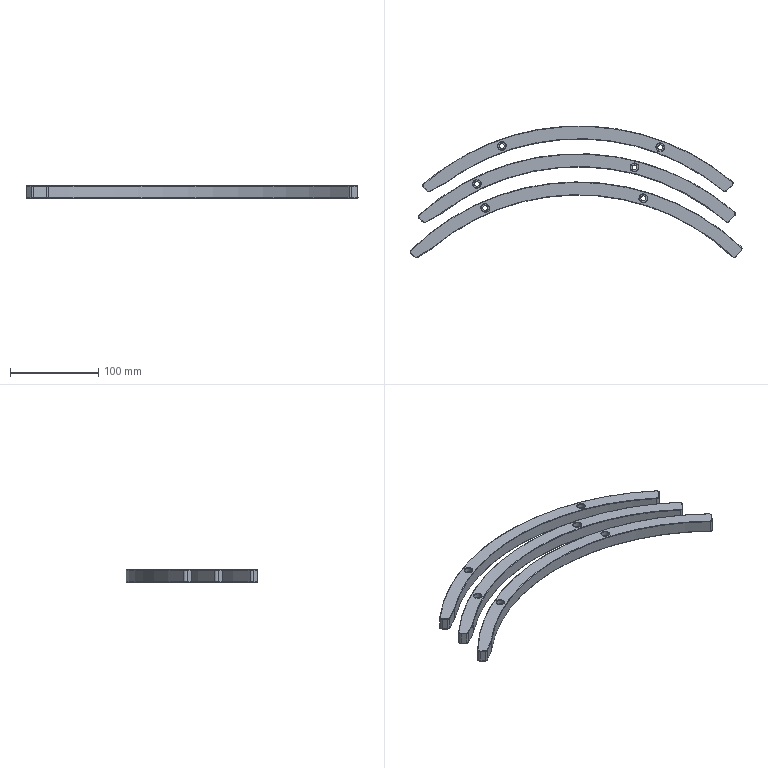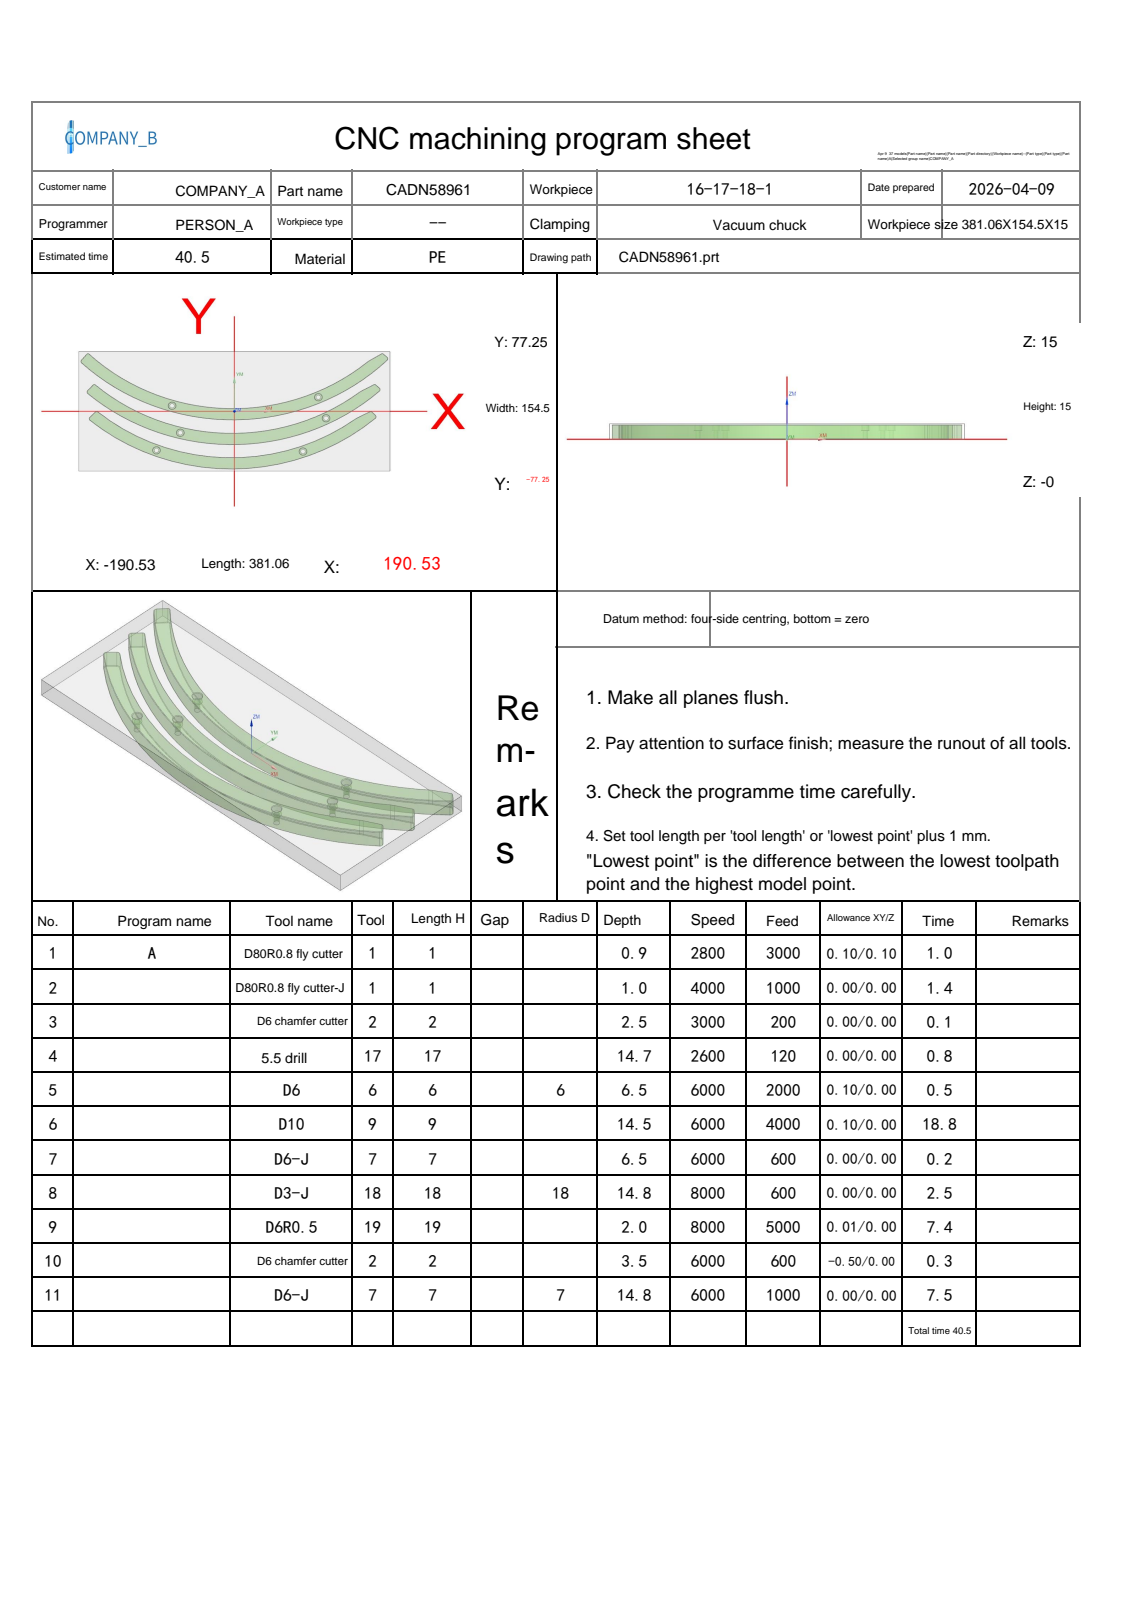NC program | NX | posted by the shop | part box 376.065 x 149.521 x 14 mm
Lines 357 to 1635 of 3929, first 1032 of 1279 lines:
N6 T09 M06
(D10  D=10. R=0. H=09 ce=0.10 di=0.00)
(MAX_Z=34. MIN_Z=0.5 Time=18.78M)
G00 G90 G54 X168.192 Y73.348 M03 S6000
G43 H09 Z34.
M08
Z14.5
G01 X177.404 Y78.848 Z14.494 F4000.
G02 X185.678 Y78.13 Z14.489 I3.64 J-6.096
G01 X190.32 Y74.13 Z14.486
G02 X191.169 Y62.707 Z14.479 I-5.287 J-6.136
X190.701 Y62.208 Z14.478 I-6.136 J5.287
X-11.247 Y-16.23 Z14.355 I-192.53 J196.5
X-190.59 Y58.586 Z14.245 I9.419 J274.939
X-191.169 Y69.766 Z14.238 I5.558 J5.892
G01 X-184.602 Y77.387 Z14.232
G02 X-174.589 Y78.131 Z14.226 I5.379 J-4.635
X-174.323 Y77.889 Z14.226 I-4.635 J-5.379
G03 X159.163 Y67.576 Z14.023 I172.494 J180.819
G02 X162.467 Y69.93 Z14.021 I16.17 J-19.197
G01 X177.404 Y78.848 Z14.011
G02 X185.678 Y78.13 Z14.006 I3.64 J-6.096
G01 X190.32 Y74.13 Z14.003
G02 X191.169 Y62.707 Z13.996 I-5.287 J-6.136
X190.701 Y62.208 Z13.996 I-6.136 J5.287
X-11.247 Y-16.23 Z13.872 I-192.53 J196.5
X-190.59 Y58.586 Z13.762 I9.419 J274.939
X-191.169 Y69.766 Z13.755 I5.558 J5.892
G01 X-184.602 Y77.387 Z13.749
G02 X-174.589 Y78.131 Z13.743 I5.379 J-4.635
X-174.323 Y77.889 Z13.743 I-4.635 J-5.379
G03 X159.163 Y67.576 Z13.54 I172.494 J180.819
G02 X162.467 Y69.93 Z13.538 I16.17 J-19.197
G01 X177.404 Y78.848 Z13.529
G02 X185.678 Y78.13 Z13.524 I3.64 J-6.096
G01 X190.32 Y74.13 Z13.52
G02 X191.169 Y62.707 Z13.513 I-5.287 J-6.136
X190.701 Y62.208 Z13.513 I-6.136 J5.287
X-11.247 Y-16.23 Z13.389 I-192.53 J196.5
X-190.59 Y58.586 Z13.279 I9.419 J274.939
X-191.169 Y69.766 Z13.272 I5.558 J5.892
G01 X-184.602 Y77.387 Z13.267
G02 X-174.589 Y78.131 Z13.26 I5.379 J-4.635
X-174.323 Y77.889 Z13.26 I-4.635 J-5.379
G03 X159.163 Y67.576 Z13.058 I172.494 J180.819
G02 X162.467 Y69.93 Z13.055 I16.17 J-19.197
G01 X177.404 Y78.848 Z13.046
G02 X185.678 Y78.13 Z13.041 I3.64 J-6.096
G01 X190.32 Y74.13 Z13.037
G02 X191.169 Y62.707 Z13.03 I-5.287 J-6.136
X190.701 Y62.208 Z13.03 I-6.136 J5.287
X-11.247 Y-16.23 Z12.907 I-192.53 J196.5
X-190.59 Y58.586 Z12.796 I9.419 J274.939
X-191.169 Y69.766 Z12.79 I5.558 J5.892
G01 X-184.602 Y77.387 Z12.784
G02 X-174.589 Y78.131 Z12.778 I5.379 J-4.635
X-174.323 Y77.889 Z12.778 I-4.635 J-5.379
G03 X159.163 Y67.576 Z12.575 I172.494 J180.819
G02 X162.467 Y69.93 Z12.573 I16.17 J-19.197
G01 X177.404 Y78.848 Z12.563
G02 X185.678 Y78.13 Z12.558 I3.64 J-6.096
G01 X190.32 Y74.13 Z12.555
G02 X191.169 Y62.707 Z12.548 I-5.287 J-6.136
X190.701 Y62.208 Z12.547 I-6.136 J5.287
X-11.247 Y-16.23 Z12.424 I-192.53 J196.5
X-190.59 Y58.586 Z12.314 I9.419 J274.939
X-191.169 Y69.766 Z12.307 I5.558 J5.892
G01 X-184.602 Y77.387 Z12.301
G02 X-174.589 Y78.131 Z12.295 I5.379 J-4.635
X-174.323 Y77.889 Z12.295 I-4.635 J-5.379
G03 X159.163 Y67.576 Z12.092 I172.494 J180.819
G02 X162.467 Y69.93 Z12.09 I16.17 J-19.197
G01 X177.404 Y78.848 Z12.08
G02 X185.678 Y78.13 Z12.075 I3.64 J-6.096
G01 X190.32 Y74.13 Z12.072
G02 X191.169 Y62.707 Z12.065 I-5.287 J-6.136
X190.701 Y62.208 Z12.065 I-6.136 J5.287
X-11.247 Y-16.23 Z11.941 I-192.53 J196.5
X-190.59 Y58.586 Z11.831 I9.419 J274.939
X-191.169 Y69.766 Z11.824 I5.558 J5.892
G01 X-184.602 Y77.387 Z11.818
G02 X-174.589 Y78.131 Z11.812 I5.379 J-4.635
X-174.323 Y77.889 Z11.812 I-4.635 J-5.379
G03 X159.163 Y67.576 Z11.609 I172.494 J180.819
G02 X162.467 Y69.93 Z11.607 I16.17 J-19.197
G01 X177.404 Y78.848 Z11.597
G02 X185.678 Y78.13 Z11.593 I3.64 J-6.096
G01 X190.32 Y74.13 Z11.589
G02 X191.169 Y62.707 Z11.582 I-5.287 J-6.136
X190.701 Y62.208 Z11.582 I-6.136 J5.287
X-11.247 Y-16.23 Z11.458 I-192.53 J196.5
X-190.59 Y58.586 Z11.348 I9.419 J274.939
X-191.169 Y69.766 Z11.341 I5.558 J5.892
G01 X-184.602 Y77.387 Z11.336
G02 X-174.589 Y78.131 Z11.329 I5.379 J-4.635
X-174.323 Y77.889 Z11.329 I-4.635 J-5.379
G03 X159.163 Y67.576 Z11.127 I172.494 J180.819
G02 X162.467 Y69.93 Z11.124 I16.17 J-19.197
G01 X177.404 Y78.848 Z11.115
G02 X185.678 Y78.13 Z11.11 I3.64 J-6.096
G01 X190.32 Y74.13 Z11.106
G02 X191.169 Y62.707 Z11.099 I-5.287 J-6.136
X190.701 Y62.208 Z11.099 I-6.136 J5.287
X-11.247 Y-16.23 Z10.975 I-192.53 J196.5
X-190.59 Y58.586 Z10.865 I9.419 J274.939
X-191.169 Y69.766 Z10.858 I5.558 J5.892
G01 X-184.602 Y77.387 Z10.853
G02 X-174.589 Y78.131 Z10.847 I5.379 J-4.635
X-174.323 Y77.889 Z10.847 I-4.635 J-5.379
G03 X159.163 Y67.576 Z10.644 I172.494 J180.819
G02 X162.467 Y69.93 Z10.642 I16.17 J-19.197
G01 X177.404 Y78.848 Z10.632
G02 X185.678 Y78.13 Z10.627 I3.64 J-6.096
G01 X190.32 Y74.13 Z10.624
G02 X191.169 Y62.707 Z10.617 I-5.287 J-6.136
X190.701 Y62.208 Z10.616 I-6.136 J5.287
X-11.247 Y-16.23 Z10.493 I-192.53 J196.5
X-190.59 Y58.586 Z10.383 I9.419 J274.939
X-191.169 Y69.766 Z10.376 I5.558 J5.892
G01 X-184.602 Y77.387 Z10.37
G02 X-174.589 Y78.131 Z10.364 I5.379 J-4.635
X-174.323 Y77.889 Z10.364 I-4.635 J-5.379
G03 X159.163 Y67.576 Z10.161 I172.494 J180.819
G02 X162.467 Y69.93 Z10.159 I16.17 J-19.197
G01 X177.404 Y78.848 Z10.149
G02 X185.678 Y78.13 Z10.144 I3.64 J-6.096
G01 X190.32 Y74.13 Z10.141
G02 X191.169 Y62.707 Z10.134 I-5.287 J-6.136
X190.701 Y62.208 Z10.133 I-6.136 J5.287
X-11.247 Y-16.23 Z10.01 I-192.53 J196.5
X-190.59 Y58.586 Z9.9 I9.419 J274.939
X-191.169 Y69.766 Z9.893 I5.558 J5.892
G01 X-184.602 Y77.387 Z9.887
G02 X-174.589 Y78.131 Z9.881 I5.379 J-4.635
X-174.323 Y77.889 Z9.881 I-4.635 J-5.379
G03 X159.163 Y67.576 Z9.678 I172.494 J180.819
G02 X162.467 Y69.93 Z9.676 I16.17 J-19.197
G01 X177.404 Y78.848 Z9.666
G02 X185.678 Y78.13 Z9.662 I3.64 J-6.096
G01 X190.32 Y74.13 Z9.658
G02 X191.169 Y62.707 Z9.651 I-5.287 J-6.136
X190.701 Y62.208 Z9.651 I-6.136 J5.287
X-11.247 Y-16.23 Z9.527 I-192.53 J196.5
X-190.59 Y58.586 Z9.417 I9.419 J274.939
X-191.169 Y69.766 Z9.41 I5.558 J5.892
G01 X-184.602 Y77.387 Z9.405
G02 X-174.589 Y78.131 Z9.398 I5.379 J-4.635
X-174.323 Y77.889 Z9.398 I-4.635 J-5.379
G03 X159.163 Y67.576 Z9.196 I172.494 J180.819
G02 X162.467 Y69.93 Z9.193 I16.17 J-19.197
G01 X177.404 Y78.848 Z9.184
G02 X185.678 Y78.13 Z9.179 I3.64 J-6.096
G01 X190.32 Y74.13 Z9.175
G02 X191.169 Y62.707 Z9.168 I-5.287 J-6.136
X190.701 Y62.208 Z9.168 I-6.136 J5.287
X-11.247 Y-16.23 Z9.044 I-192.53 J196.5
X-190.59 Y58.586 Z8.934 I9.419 J274.939
X-191.169 Y69.766 Z8.927 I5.558 J5.892
G01 X-184.602 Y77.387 Z8.922
G02 X-174.589 Y78.131 Z8.916 I5.379 J-4.635
X-174.323 Y77.889 Z8.915 I-4.635 J-5.379
G03 X159.163 Y67.576 Z8.713 I172.494 J180.819
G02 X162.467 Y69.93 Z8.711 I16.17 J-19.197
G01 X177.404 Y78.848 Z8.701
G02 X185.678 Y78.13 Z8.696 I3.64 J-6.096
G01 X190.32 Y74.13 Z8.693
G02 X191.169 Y62.707 Z8.686 I-5.287 J-6.136
X190.701 Y62.208 Z8.685 I-6.136 J5.287
X-11.247 Y-16.23 Z8.562 I-192.53 J196.5
X-190.59 Y58.586 Z8.452 I9.419 J274.939
X-191.169 Y69.766 Z8.445 I5.558 J5.892
G01 X-184.602 Y77.387 Z8.439
G02 X-174.589 Y78.131 Z8.433 I5.379 J-4.635
X-174.323 Y77.889 Z8.433 I-4.635 J-5.379
G03 X159.163 Y67.576 Z8.23 I172.494 J180.819
G02 X162.467 Y69.93 Z8.228 I16.17 J-19.197
G01 X177.404 Y78.848 Z8.218
G02 X185.678 Y78.13 Z8.213 I3.64 J-6.096
G01 X190.32 Y74.13 Z8.21
G02 X191.169 Y62.707 Z8.203 I-5.287 J-6.136
X190.701 Y62.208 Z8.202 I-6.136 J5.287
X-11.247 Y-16.23 Z8.079 I-192.53 J196.5
X-190.59 Y58.586 Z7.969 I9.419 J274.939
X-191.169 Y69.766 Z7.962 I5.558 J5.892
G01 X-184.602 Y77.387 Z7.956
G02 X-174.589 Y78.131 Z7.95 I5.379 J-4.635
X-174.323 Y77.889 Z7.95 I-4.635 J-5.379
G03 X159.163 Y67.576 Z7.747 I172.494 J180.819
G02 X162.467 Y69.93 Z7.745 I16.17 J-19.197
G01 X177.404 Y78.848 Z7.735
G02 X185.678 Y78.13 Z7.731 I3.64 J-6.096
G01 X190.32 Y74.13 Z7.727
G02 X191.169 Y62.707 Z7.72 I-5.287 J-6.136
X190.701 Y62.208 Z7.72 I-6.136 J5.287
X-11.247 Y-16.23 Z7.596 I-192.53 J196.5
X-190.59 Y58.586 Z7.486 I9.419 J274.939
X-191.169 Y69.766 Z7.479 I5.558 J5.892
G01 X-184.602 Y77.387 Z7.474
G02 X-174.589 Y78.131 Z7.467 I5.379 J-4.635
X-174.323 Y77.889 Z7.467 I-4.635 J-5.379
G03 X159.163 Y67.576 Z7.265 I172.494 J180.819
G02 X162.467 Y69.93 Z7.262 I16.17 J-19.197
G01 X177.404 Y78.848 Z7.253
G02 X185.678 Y78.13 Z7.248 I3.64 J-6.096
G01 X190.32 Y74.13 Z7.244
G02 X191.169 Y62.707 Z7.237 I-5.287 J-6.136
X190.701 Y62.208 Z7.237 I-6.136 J5.287
X-11.247 Y-16.23 Z7.113 I-192.53 J196.5
X-190.59 Y58.586 Z7.003 I9.419 J274.939
X-191.169 Y69.766 Z6.996 I5.558 J5.892
G01 X-184.602 Y77.387 Z6.991
G02 X-174.589 Y78.131 Z6.985 I5.379 J-4.635
X-174.323 Y77.889 Z6.984 I-4.635 J-5.379
G03 X159.163 Y67.576 Z6.782 I172.494 J180.819
G02 X162.467 Y69.93 Z6.78 I16.17 J-19.197
G01 X177.404 Y78.848 Z6.77
G02 X185.678 Y78.13 Z6.765 I3.64 J-6.096
G01 X190.32 Y74.13 Z6.762
G02 X191.169 Y62.707 Z6.755 I-5.287 J-6.136
X190.701 Y62.208 Z6.754 I-6.136 J5.287
X-11.247 Y-16.23 Z6.631 I-192.53 J196.5
X-190.59 Y58.586 Z6.52 I9.419 J274.939
X-191.169 Y69.766 Z6.514 I5.558 J5.892
G01 X-184.602 Y77.387 Z6.508
G02 X-174.589 Y78.131 Z6.502 I5.379 J-4.635
X-174.323 Y77.889 Z6.502 I-4.635 J-5.379
G03 X159.163 Y67.576 Z6.299 I172.494 J180.819
G02 X162.467 Y69.93 Z6.297 I16.17 J-19.197
G01 X177.404 Y78.848 Z6.287
G02 X185.678 Y78.13 Z6.282 I3.64 J-6.096
G01 X190.32 Y74.13 Z6.279
G02 X191.169 Y62.707 Z6.272 I-5.287 J-6.136
X190.701 Y62.208 Z6.271 I-6.136 J5.287
X-11.247 Y-16.23 Z6.148 I-192.53 J196.5
X-190.59 Y58.586 Z6.038 I9.419 J274.939
X-191.169 Y69.766 Z6.031 I5.558 J5.892
G01 X-184.602 Y77.387 Z6.025
G02 X-174.589 Y78.131 Z6.019 I5.379 J-4.635
X-174.323 Y77.889 Z6.019 I-4.635 J-5.379
G03 X159.163 Y67.576 Z5.816 I172.494 J180.819
G02 X162.467 Y69.93 Z5.814 I16.17 J-19.197
G01 X177.404 Y78.848 Z5.804
G02 X185.678 Y78.13 Z5.799 I3.64 J-6.096
G01 X190.32 Y74.13 Z5.796
G02 X191.169 Y62.707 Z5.789 I-5.287 J-6.136
X190.701 Y62.208 Z5.789 I-6.136 J5.287
X-11.247 Y-16.23 Z5.665 I-192.53 J196.5
X-190.59 Y58.586 Z5.555 I9.419 J274.939
X-191.169 Y69.766 Z5.548 I5.558 J5.892
G01 X-184.602 Y77.387 Z5.543
G02 X-174.589 Y78.131 Z5.536 I5.379 J-4.635
X-174.323 Y77.889 Z5.536 I-4.635 J-5.379
G03 X159.163 Y67.576 Z5.334 I172.494 J180.819
G02 X162.467 Y69.93 Z5.331 I16.17 J-19.197
G01 X177.404 Y78.848 Z5.322
G02 X185.678 Y78.13 Z5.317 I3.64 J-6.096
G01 X190.32 Y74.13 Z5.313
G02 X191.169 Y62.707 Z5.306 I-5.287 J-6.136
X190.701 Y62.208 Z5.306 I-6.136 J5.287
X-11.247 Y-16.23 Z5.182 I-192.53 J196.5
X-190.59 Y58.586 Z5.072 I9.419 J274.939
X-191.169 Y69.766 Z5.065 I5.558 J5.892
G01 X-184.602 Y77.387 Z5.06
G02 X-174.589 Y78.131 Z5.054 I5.379 J-4.635
X-174.323 Y77.889 Z5.053 I-4.635 J-5.379
G03 X159.163 Y67.576 Z4.851 I172.494 J180.819
G02 X162.467 Y69.93 Z4.849 I16.17 J-19.197
G01 X177.404 Y78.848 Z4.839
G02 X185.678 Y78.13 Z4.834 I3.64 J-6.096
G01 X190.32 Y74.13 Z4.831
G02 X191.169 Y62.707 Z4.824 I-5.287 J-6.136
X190.701 Y62.208 Z4.823 I-6.136 J5.287
X-11.247 Y-16.23 Z4.7 I-192.53 J196.5
X-190.59 Y58.586 Z4.589 I9.419 J274.939
X-191.169 Y69.766 Z4.583 I5.558 J5.892
G01 X-184.602 Y77.387 Z4.577
G02 X-174.589 Y78.131 Z4.571 I5.379 J-4.635
X-174.323 Y77.889 Z4.571 I-4.635 J-5.379
G03 X159.163 Y67.576 Z4.368 I172.494 J180.819
G02 X162.467 Y69.93 Z4.366 I16.17 J-19.197
G01 X177.404 Y78.848 Z4.356
G02 X185.678 Y78.13 Z4.351 I3.64 J-6.096
G01 X190.32 Y74.13 Z4.348
G02 X191.169 Y62.707 Z4.341 I-5.287 J-6.136
X190.701 Y62.208 Z4.34 I-6.136 J5.287
X-11.247 Y-16.23 Z4.217 I-192.53 J196.5
X-190.59 Y58.586 Z4.107 I9.419 J274.939
X-191.169 Y69.766 Z4.1 I5.558 J5.892
G01 X-184.602 Y77.387 Z4.094
G02 X-174.589 Y78.131 Z4.088 I5.379 J-4.635
X-174.323 Y77.889 Z4.088 I-4.635 J-5.379
G03 X159.163 Y67.576 Z3.885 I172.494 J180.819
G02 X162.467 Y69.93 Z3.883 I16.17 J-19.197
G01 X177.404 Y78.848 Z3.873
G02 X185.678 Y78.13 Z3.868 I3.64 J-6.096
G01 X190.32 Y74.13 Z3.865
G02 X191.169 Y62.707 Z3.858 I-5.287 J-6.136
X190.701 Y62.208 Z3.858 I-6.136 J5.287
X-11.247 Y-16.23 Z3.734 I-192.53 J196.5
X-190.59 Y58.586 Z3.624 I9.419 J274.939
X-191.169 Y69.766 Z3.617 I5.558 J5.892
G01 X-184.602 Y77.387 Z3.612
G02 X-174.589 Y78.131 Z3.605 I5.379 J-4.635
X-174.323 Y77.889 Z3.605 I-4.635 J-5.379
G03 X159.163 Y67.576 Z3.403 I172.494 J180.819
G02 X162.467 Y69.93 Z3.4 I16.17 J-19.197
G01 X177.404 Y78.848 Z3.391
G02 X185.678 Y78.13 Z3.386 I3.64 J-6.096
G01 X190.32 Y74.13 Z3.382
G02 X191.169 Y62.707 Z3.375 I-5.287 J-6.136
X190.701 Y62.208 Z3.375 I-6.136 J5.287
X-11.247 Y-16.23 Z3.251 I-192.53 J196.5
X-190.59 Y58.586 Z3.141 I9.419 J274.939
X-191.169 Y69.766 Z3.134 I5.558 J5.892
G01 X-184.602 Y77.387 Z3.129
G02 X-174.589 Y78.131 Z3.123 I5.379 J-4.635
X-174.323 Y77.889 Z3.122 I-4.635 J-5.379
G03 X159.163 Y67.576 Z2.92 I172.494 J180.819
G02 X162.467 Y69.93 Z2.917 I16.17 J-19.197
G01 X177.404 Y78.848 Z2.908
G02 X185.678 Y78.13 Z2.903 I3.64 J-6.096
G01 X190.32 Y74.13 Z2.9
G02 X191.169 Y62.707 Z2.892 I-5.287 J-6.136
X190.701 Y62.208 Z2.892 I-6.136 J5.287
X-11.247 Y-16.23 Z2.769 I-192.53 J196.5
X-190.59 Y58.586 Z2.658 I9.419 J274.939
X-191.169 Y69.766 Z2.652 I5.558 J5.892
G01 X-184.602 Y77.387 Z2.646
G02 X-174.589 Y78.131 Z2.64 I5.379 J-4.635
X-174.323 Y77.889 Z2.64 I-4.635 J-5.379
G03 X159.163 Y67.576 Z2.437 I172.494 J180.819
G02 X162.467 Y69.93 Z2.435 I16.17 J-19.197
G01 X177.404 Y78.848 Z2.425
G02 X185.678 Y78.13 Z2.42 I3.64 J-6.096
G01 X190.32 Y74.13 Z2.417
G02 X191.169 Y62.707 Z2.41 I-5.287 J-6.136
X190.701 Y62.208 Z2.409 I-6.136 J5.287
X-11.247 Y-16.23 Z2.286 I-192.53 J196.5
X-190.59 Y58.586 Z2.176 I9.419 J274.939
X-191.169 Y69.766 Z2.169 I5.558 J5.892
G01 X-184.602 Y77.387 Z2.163
G02 X-174.589 Y78.131 Z2.157 I5.379 J-4.635
X-174.323 Y77.889 Z2.157 I-4.635 J-5.379
G03 X159.163 Y67.576 Z1.954 I172.494 J180.819
G02 X162.467 Y69.93 Z1.952 I16.17 J-19.197
G01 X177.404 Y78.848 Z1.942
G02 X185.678 Y78.13 Z1.937 I3.64 J-6.096
G01 X190.32 Y74.13 Z1.934
G02 X191.169 Y62.707 Z1.927 I-5.287 J-6.136
X190.701 Y62.208 Z1.927 I-6.136 J5.287
X-11.247 Y-16.23 Z1.803 I-192.53 J196.5
X-190.59 Y58.586 Z1.693 I9.419 J274.939
X-191.169 Y69.766 Z1.686 I5.558 J5.892
G01 X-184.602 Y77.387 Z1.68
G02 X-174.589 Y78.131 Z1.674 I5.379 J-4.635
X-174.323 Y77.889 Z1.674 I-4.635 J-5.379
G03 X159.163 Y67.576 Z1.471 I172.494 J180.819
G02 X162.467 Y69.93 Z1.469 I16.17 J-19.197
G01 X177.404 Y78.848 Z1.46
G02 X185.678 Y78.13 Z1.455 I3.64 J-6.096
G01 X190.32 Y74.13 Z1.451
G02 X191.169 Y62.707 Z1.444 I-5.287 J-6.136
X190.701 Y62.208 Z1.444 I-6.136 J5.287
X-11.247 Y-16.23 Z1.32 I-192.53 J196.5
X-190.59 Y58.586 Z1.21 I9.419 J274.939
X-191.169 Y69.766 Z1.203 I5.558 J5.892
G01 X-184.602 Y77.387 Z1.198
G02 X-174.589 Y78.131 Z1.192 I5.379 J-4.635
X-174.323 Y77.889 Z1.191 I-4.635 J-5.379
G03 X159.163 Y67.576 Z.989 I172.494 J180.819
G02 X162.467 Y69.93 Z.986 I16.17 J-19.197
G01 X177.404 Y78.848 Z.977
G02 X185.678 Y78.13 Z.972 I3.64 J-6.096
G01 X190.32 Y74.13 Z.968
G02 X191.169 Y62.707 Z.961 I-5.287 J-6.136
X190.701 Y62.208 Z.961 I-6.136 J5.287
X-11.247 Y-16.23 Z.838 I-192.53 J196.5
X-190.59 Y58.586 Z.727 I9.419 J274.939
X-191.169 Y69.766 Z.721 I5.558 J5.892
G01 X-184.602 Y77.387 Z.715
G02 X-174.589 Y78.131 Z.709 I5.379 J-4.635
X-174.323 Y77.889 Z.709 I-4.635 J-5.379
G03 X159.163 Y67.576 Z.506 I172.494 J180.819
G02 X162.467 Y69.93 Z.504 I16.17 J-19.197
G01 X168.192 Y73.348 Z.5
X177.404 Y78.848
G02 X181.043 Y79.851 I3.64 J-6.096
X185.678 Y78.13 I0.0 J-7.1
G01 X190.32 Y74.13
G02 X193.132 Y67.994 I-5.287 J-6.136
X190.701 Y62.208 I-8.1 J0.0
X-1.828 Y-16.391 I-192.53 J196.5
X-190.59 Y58.586 I0.0 J275.1
X-193.132 Y64.479 I5.558 J5.892
X-191.169 Y69.766 I8.1 J0.0
G01 X-184.602 Y77.387
G02 X-179.224 Y79.852 I5.379 J-4.635
X-174.589 Y78.131 I0.0 J-7.1
X-174.323 Y77.889 I-4.635 J-5.379
G03 X-1.828 Y8.809 I172.494 J180.819
X159.163 Y67.576 I0.0 J249.9
G02 X162.467 Y69.93 I16.17 J-19.197
G01 X168.192 Y73.348
X168.621 Y73.604
Z1.5
G00 Z34.
X154.201 Y-.583
Z14.5
G01 X163.737 Y4.31 Z14.494
G02 X171.976 Y3.036 Z14.488 I3.241 J-6.317
G01 X176.33 Y-1.28 Z14.485
G02 X176.382 Y-12.735 Z14.477 I-5.702 J-5.753
X175.916 Y-13.17 Z14.477 I-5.753 J5.702
X-180.14 Y-15.773 Z14.244 I-179.561 J208.418
X-181.156 Y-4.363 Z14.236 I5.197 J6.213
X-180.696 Y-3.858 Z14.236 I6.213 J-5.197
G01 X-174.337 Y2.559 Z14.23
G02 X-163.406 Y3.085 Z14.223 I5.753 J-5.702
G03 X144.832 Y-5.761 Z14.024 I159.761 J192.163
G02 X148.286 Y-3.618 Z14.021 I14.913 J-20.189
G01 X163.737 Y4.31 Z14.011
G02 X171.976 Y3.036 Z14.005 I3.241 J-6.317
G01 X176.33 Y-1.28 Z14.002
G02 X176.382 Y-12.735 Z13.994 I-5.702 J-5.753
X175.916 Y-13.17 Z13.994 I-5.753 J5.702
X-180.14 Y-15.773 Z13.761 I-179.561 J208.418
X-181.156 Y-4.363 Z13.754 I5.197 J6.213
X-180.696 Y-3.858 Z13.753 I6.213 J-5.197
G01 X-174.337 Y2.559 Z13.748
G02 X-163.406 Y3.085 Z13.74 I5.753 J-5.702
G03 X144.832 Y-5.761 Z13.541 I159.761 J192.163
G02 X148.286 Y-3.618 Z13.538 I14.913 J-20.189
G01 X163.737 Y4.31 Z13.528
G02 X171.976 Y3.036 Z13.523 I3.241 J-6.317
G01 X176.33 Y-1.28 Z13.519
G02 X176.382 Y-12.735 Z13.511 I-5.702 J-5.753
X175.916 Y-13.17 Z13.511 I-5.753 J5.702
X-180.14 Y-15.773 Z13.278 I-179.561 J208.418
X-181.156 Y-4.363 Z13.271 I5.197 J6.213
X-180.696 Y-3.858 Z13.27 I6.213 J-5.197
G01 X-174.337 Y2.559 Z13.265
G02 X-163.406 Y3.085 Z13.258 I5.753 J-5.702
G03 X144.832 Y-5.761 Z13.058 I159.761 J192.163
G02 X148.286 Y-3.618 Z13.056 I14.913 J-20.189
G01 X163.737 Y4.31 Z13.045
G02 X171.976 Y3.036 Z13.04 I3.241 J-6.317
G01 X176.33 Y-1.28 Z13.036
G02 X176.382 Y-12.735 Z13.029 I-5.702 J-5.753
X175.916 Y-13.17 Z13.028 I-5.753 J5.702
X-180.14 Y-15.773 Z12.796 I-179.561 J208.418
X-181.156 Y-4.363 Z12.788 I5.197 J6.213
X-180.696 Y-3.858 Z12.788 I6.213 J-5.197
G01 X-174.337 Y2.559 Z12.782
G02 X-163.406 Y3.085 Z12.775 I5.753 J-5.702
G03 X144.832 Y-5.761 Z12.575 I159.761 J192.163
G02 X148.286 Y-3.618 Z12.573 I14.913 J-20.189
G01 X163.737 Y4.31 Z12.563
G02 X171.976 Y3.036 Z12.557 I3.241 J-6.317
G01 X176.33 Y-1.28 Z12.553
G02 X176.382 Y-12.735 Z12.546 I-5.702 J-5.753
X175.916 Y-13.17 Z12.545 I-5.753 J5.702
X-180.14 Y-15.773 Z12.313 I-179.561 J208.418
X-181.156 Y-4.363 Z12.305 I5.197 J6.213
X-180.696 Y-3.858 Z12.305 I6.213 J-5.197
G01 X-174.337 Y2.559 Z12.299
G02 X-163.406 Y3.085 Z12.292 I5.753 J-5.702
G03 X144.832 Y-5.761 Z12.093 I159.761 J192.163
G02 X148.286 Y-3.618 Z12.09 I14.913 J-20.189
G01 X163.737 Y4.31 Z12.08
G02 X171.976 Y3.036 Z12.074 I3.241 J-6.317
G01 X176.33 Y-1.28 Z12.071
G02 X176.382 Y-12.735 Z12.063 I-5.702 J-5.753
X175.916 Y-13.17 Z12.063 I-5.753 J5.702
X-180.14 Y-15.773 Z11.83 I-179.561 J208.418
X-181.156 Y-4.363 Z11.823 I5.197 J6.213
X-180.696 Y-3.858 Z11.822 I6.213 J-5.197
G01 X-174.337 Y2.559 Z11.817
G02 X-163.406 Y3.085 Z11.809 I5.753 J-5.702
G03 X144.832 Y-5.761 Z11.61 I159.761 J192.163
G02 X148.286 Y-3.618 Z11.607 I14.913 J-20.189
G01 X163.737 Y4.31 Z11.597
G02 X171.976 Y3.036 Z11.592 I3.241 J-6.317
G01 X176.33 Y-1.28 Z11.588
G02 X176.382 Y-12.735 Z11.58 I-5.702 J-5.753
X175.916 Y-13.17 Z11.58 I-5.753 J5.702
X-180.14 Y-15.773 Z11.347 I-179.561 J208.418
X-181.156 Y-4.363 Z11.34 I5.197 J6.213
X-180.696 Y-3.858 Z11.339 I6.213 J-5.197
G01 X-174.337 Y2.559 Z11.334
G02 X-163.406 Y3.085 Z11.327 I5.753 J-5.702
G03 X144.832 Y-5.761 Z11.127 I159.761 J192.163
G02 X148.286 Y-3.618 Z11.125 I14.913 J-20.189
G01 X163.737 Y4.31 Z11.114
G02 X171.976 Y3.036 Z11.109 I3.241 J-6.317
G01 X176.33 Y-1.28 Z11.105
G02 X176.382 Y-12.735 Z11.098 I-5.702 J-5.753
X175.916 Y-13.17 Z11.097 I-5.753 J5.702
X-180.14 Y-15.773 Z10.865 I-179.561 J208.418
X-181.156 Y-4.363 Z10.857 I5.197 J6.213
X-180.696 Y-3.858 Z10.857 I6.213 J-5.197
G01 X-174.337 Y2.559 Z10.851
G02 X-163.406 Y3.085 Z10.844 I5.753 J-5.702
G03 X144.832 Y-5.761 Z10.644 I159.761 J192.163
G02 X148.286 Y-3.618 Z10.642 I14.913 J-20.189
G01 X163.737 Y4.31 Z10.631
G02 X171.976 Y3.036 Z10.626 I3.241 J-6.317
G01 X176.33 Y-1.28 Z10.622
G02 X176.382 Y-12.735 Z10.615 I-5.702 J-5.753
X175.916 Y-13.17 Z10.614 I-5.753 J5.702
X-180.14 Y-15.773 Z10.382 I-179.561 J208.418
X-181.156 Y-4.363 Z10.374 I5.197 J6.213
X-180.696 Y-3.858 Z10.374 I6.213 J-5.197
G01 X-174.337 Y2.559 Z10.368
G02 X-163.406 Y3.085 Z10.361 I5.753 J-5.702
G03 X144.832 Y-5.761 Z10.162 I159.761 J192.163
G02 X148.286 Y-3.618 Z10.159 I14.913 J-20.189
G01 X163.737 Y4.31 Z10.149
G02 X171.976 Y3.036 Z10.143 I3.241 J-6.317
G01 X176.33 Y-1.28 Z10.14
G02 X176.382 Y-12.735 Z10.132 I-5.702 J-5.753
X175.916 Y-13.17 Z10.132 I-5.753 J5.702
X-180.14 Y-15.773 Z9.899 I-179.561 J208.418
X-181.156 Y-4.363 Z9.891 I5.197 J6.213
X-180.696 Y-3.858 Z9.891 I6.213 J-5.197
G01 X-174.337 Y2.559 Z9.886
G02 X-163.406 Y3.085 Z9.878 I5.753 J-5.702
G03 X144.832 Y-5.761 Z9.679 I159.761 J192.163
G02 X148.286 Y-3.618 Z9.676 I14.913 J-20.189
G01 X163.737 Y4.31 Z9.666
G02 X171.976 Y3.036 Z9.661 I3.241 J-6.317
G01 X176.33 Y-1.28 Z9.657
G02 X176.382 Y-12.735 Z9.649 I-5.702 J-5.753
X175.916 Y-13.17 Z9.649 I-5.753 J5.702
X-180.14 Y-15.773 Z9.416 I-179.561 J208.418
X-181.156 Y-4.363 Z9.409 I5.197 J6.213
X-180.696 Y-3.858 Z9.408 I6.213 J-5.197
G01 X-174.337 Y2.559 Z9.403
G02 X-163.406 Y3.085 Z9.396 I5.753 J-5.702
G03 X144.832 Y-5.761 Z9.196 I159.761 J192.163
G02 X148.286 Y-3.618 Z9.194 I14.913 J-20.189
G01 X163.737 Y4.31 Z9.183
G02 X171.976 Y3.036 Z9.178 I3.241 J-6.317
G01 X176.33 Y-1.28 Z9.174
G02 X176.382 Y-12.735 Z9.167 I-5.702 J-5.753
X175.916 Y-13.17 Z9.166 I-5.753 J5.702
X-180.14 Y-15.773 Z8.934 I-179.561 J208.418
X-181.156 Y-4.363 Z8.926 I5.197 J6.213
X-180.696 Y-3.858 Z8.926 I6.213 J-5.197
G01 X-174.337 Y2.559 Z8.92
G02 X-163.406 Y3.085 Z8.913 I5.753 J-5.702
G03 X144.832 Y-5.761 Z8.713 I159.761 J192.163
G02 X148.286 Y-3.618 Z8.711 I14.913 J-20.189
G01 X163.737 Y4.31 Z8.7
G02 X171.976 Y3.036 Z8.695 I3.241 J-6.317
G01 X176.33 Y-1.28 Z8.691
G02 X176.382 Y-12.735 Z8.684 I-5.702 J-5.753
X175.916 Y-13.17 Z8.683 I-5.753 J5.702
X-180.14 Y-15.773 Z8.451 I-179.561 J208.418
X-181.156 Y-4.363 Z8.443 I5.197 J6.213
X-180.696 Y-3.858 Z8.443 I6.213 J-5.197
G01 X-174.337 Y2.559 Z8.437
G02 X-163.406 Y3.085 Z8.43 I5.753 J-5.702
G03 X144.832 Y-5.761 Z8.231 I159.761 J192.163
G02 X148.286 Y-3.618 Z8.228 I14.913 J-20.189
G01 X163.737 Y4.31 Z8.218
G02 X171.976 Y3.036 Z8.212 I3.241 J-6.317
G01 X176.33 Y-1.28 Z8.209
G02 X176.382 Y-12.735 Z8.201 I-5.702 J-5.753
X175.916 Y-13.17 Z8.201 I-5.753 J5.702
X-180.14 Y-15.773 Z7.968 I-179.561 J208.418
X-181.156 Y-4.363 Z7.96 I5.197 J6.213
X-180.696 Y-3.858 Z7.96 I6.213 J-5.197
G01 X-174.337 Y2.559 Z7.955
G02 X-163.406 Y3.085 Z7.947 I5.753 J-5.702
G03 X144.832 Y-5.761 Z7.748 I159.761 J192.163
G02 X148.286 Y-3.618 Z7.745 I14.913 J-20.189
G01 X163.737 Y4.31 Z7.735
G02 X171.976 Y3.036 Z7.73 I3.241 J-6.317
G01 X176.33 Y-1.28 Z7.726
G02 X176.382 Y-12.735 Z7.718 I-5.702 J-5.753
X175.916 Y-13.17 Z7.718 I-5.753 J5.702
X-180.14 Y-15.773 Z7.485 I-179.561 J208.418
X-181.156 Y-4.363 Z7.478 I5.197 J6.213
X-180.696 Y-3.858 Z7.477 I6.213 J-5.197
G01 X-174.337 Y2.559 Z7.472
G02 X-163.406 Y3.085 Z7.465 I5.753 J-5.702
G03 X144.832 Y-5.761 Z7.265 I159.761 J192.163
G02 X148.286 Y-3.618 Z7.263 I14.913 J-20.189
G01 X163.737 Y4.31 Z7.252
G02 X171.976 Y3.036 Z7.247 I3.241 J-6.317
G01 X176.33 Y-1.28 Z7.243
G02 X176.382 Y-12.735 Z7.236 I-5.702 J-5.753
X175.916 Y-13.17 Z7.235 I-5.753 J5.702
X-180.14 Y-15.773 Z7.003 I-179.561 J208.418
X-181.156 Y-4.363 Z6.995 I5.197 J6.213
X-180.696 Y-3.858 Z6.995 I6.213 J-5.197
G01 X-174.337 Y2.559 Z6.989
G02 X-163.406 Y3.085 Z6.982 I5.753 J-5.702
G03 X144.832 Y-5.761 Z6.782 I159.761 J192.163
G02 X148.286 Y-3.618 Z6.78 I14.913 J-20.189
G01 X163.737 Y4.31 Z6.769
G02 X171.976 Y3.036 Z6.764 I3.241 J-6.317
G01 X176.33 Y-1.28 Z6.76
G02 X176.382 Y-12.735 Z6.753 I-5.702 J-5.753
X175.916 Y-13.17 Z6.752 I-5.753 J5.702
X-180.14 Y-15.773 Z6.52 I-179.561 J208.418
X-181.156 Y-4.363 Z6.512 I5.197 J6.213
X-180.696 Y-3.858 Z6.512 I6.213 J-5.197
G01 X-174.337 Y2.559 Z6.506
G02 X-163.406 Y3.085 Z6.499 I5.753 J-5.702
G03 X144.832 Y-5.761 Z6.3 I159.761 J192.163
G02 X148.286 Y-3.618 Z6.297 I14.913 J-20.189
G01 X163.737 Y4.31 Z6.287
G02 X171.976 Y3.036 Z6.281 I3.241 J-6.317
G01 X176.33 Y-1.28 Z6.278
G02 X176.382 Y-12.735 Z6.27 I-5.702 J-5.753
X175.916 Y-13.17 Z6.27 I-5.753 J5.702
X-180.14 Y-15.773 Z6.037 I-179.561 J208.418
X-181.156 Y-4.363 Z6.029 I5.197 J6.213
X-180.696 Y-3.858 Z6.029 I6.213 J-5.197
G01 X-174.337 Y2.559 Z6.024
G02 X-163.406 Y3.085 Z6.016 I5.753 J-5.702
G03 X144.832 Y-5.761 Z5.817 I159.761 J192.163
G02 X148.286 Y-3.618 Z5.814 I14.913 J-20.189
G01 X163.737 Y4.31 Z5.804
G02 X171.976 Y3.036 Z5.799 I3.241 J-6.317
G01 X176.33 Y-1.28 Z5.795
G02 X176.382 Y-12.735 Z5.787 I-5.702 J-5.753
X175.916 Y-13.17 Z5.787 I-5.753 J5.702
X-180.14 Y-15.773 Z5.554 I-179.561 J208.418
X-181.156 Y-4.363 Z5.547 I5.197 J6.213
X-180.696 Y-3.858 Z5.546 I6.213 J-5.197
G01 X-174.337 Y2.559 Z5.541
G02 X-163.406 Y3.085 Z5.534 I5.753 J-5.702
G03 X144.832 Y-5.761 Z5.334 I159.761 J192.163
G02 X148.286 Y-3.618 Z5.332 I14.913 J-20.189
G01 X163.737 Y4.31 Z5.321
G02 X171.976 Y3.036 Z5.316 I3.241 J-6.317
G01 X176.33 Y-1.28 Z5.312
G02 X176.382 Y-12.735 Z5.304 I-5.702 J-5.753
X175.916 Y-13.17 Z5.304 I-5.753 J5.702
X-180.14 Y-15.773 Z5.072 I-179.561 J208.418
X-181.156 Y-4.363 Z5.064 I5.197 J6.213
X-180.696 Y-3.858 Z5.063 I6.213 J-5.197
G01 X-174.337 Y2.559 Z5.058
G02 X-163.406 Y3.085 Z5.051 I5.753 J-5.702
G03 X144.832 Y-5.761 Z4.851 I159.761 J192.163
G02 X148.286 Y-3.618 Z4.849 I14.913 J-20.189
G01 X163.737 Y4.31 Z4.838
G02 X171.976 Y3.036 Z4.833 I3.241 J-6.317
G01 X176.33 Y-1.28 Z4.829
G02 X176.382 Y-12.735 Z4.822 I-5.702 J-5.753
X175.916 Y-13.17 Z4.821 I-5.753 J5.702
X-180.14 Y-15.773 Z4.589 I-179.561 J208.418
X-181.156 Y-4.363 Z4.581 I5.197 J6.213
X-180.696 Y-3.858 Z4.581 I6.213 J-5.197
G01 X-174.337 Y2.559 Z4.575
G02 X-163.406 Y3.085 Z4.568 I5.753 J-5.702
G03 X144.832 Y-5.761 Z4.369 I159.761 J192.163
G02 X148.286 Y-3.618 Z4.366 I14.913 J-20.189
G01 X163.737 Y4.31 Z4.356
G02 X171.976 Y3.036 Z4.35 I3.241 J-6.317
G01 X176.33 Y-1.28 Z4.347
G02 X176.382 Y-12.735 Z4.339 I-5.702 J-5.753
X175.916 Y-13.17 Z4.339 I-5.753 J5.702
X-180.14 Y-15.773 Z4.106 I-179.561 J208.418
X-181.156 Y-4.363 Z4.098 I5.197 J6.213
X-180.696 Y-3.858 Z4.098 I6.213 J-5.197
G01 X-174.337 Y2.559 Z4.093
G02 X-163.406 Y3.085 Z4.085 I5.753 J-5.702
G03 X144.832 Y-5.761 Z3.886 I159.761 J192.163
G02 X148.286 Y-3.618 Z3.883 I14.913 J-20.189
G01 X163.737 Y4.31 Z3.873
G02 X171.976 Y3.036 Z3.868 I3.241 J-6.317
G01 X176.33 Y-1.28 Z3.864
G02 X176.382 Y-12.735 Z3.856 I-5.702 J-5.753
X175.916 Y-13.17 Z3.856 I-5.753 J5.702
X-180.14 Y-15.773 Z3.623 I-179.561 J208.418
X-181.156 Y-4.363 Z3.616 I5.197 J6.213
X-180.696 Y-3.858 Z3.615 I6.213 J-5.197
G01 X-174.337 Y2.559 Z3.61
G02 X-163.406 Y3.085 Z3.603 I5.753 J-5.702
G03 X144.832 Y-5.761 Z3.403 I159.761 J192.163
G02 X148.286 Y-3.618 Z3.401 I14.913 J-20.189
G01 X163.737 Y4.31 Z3.39
G02 X171.976 Y3.036 Z3.385 I3.241 J-6.317
G01 X176.33 Y-1.28 Z3.381
G02 X176.382 Y-12.735 Z3.373 I-5.702 J-5.753
X175.916 Y-13.17 Z3.373 I-5.753 J5.702
X-180.14 Y-15.773 Z3.14 I-179.561 J208.418
X-181.156 Y-4.363 Z3.133 I5.197 J6.213
X-180.696 Y-3.858 Z3.132 I6.213 J-5.197
G01 X-174.337 Y2.559 Z3.127
G02 X-163.406 Y3.085 Z3.12 I5.753 J-5.702
G03 X144.832 Y-5.761 Z2.92 I159.761 J192.163
G02 X148.286 Y-3.618 Z2.918 I14.913 J-20.189
G01 X163.737 Y4.31 Z2.907
G02 X171.976 Y3.036 Z2.902 I3.241 J-6.317
G01 X176.33 Y-1.28 Z2.898
G02 X176.382 Y-12.735 Z2.891 I-5.702 J-5.753
X175.916 Y-13.17 Z2.89 I-5.753 J5.702
X-180.14 Y-15.773 Z2.658 I-179.561 J208.418
X-181.156 Y-4.363 Z2.65 I5.197 J6.213
X-180.696 Y-3.858 Z2.65 I6.213 J-5.197
G01 X-174.337 Y2.559 Z2.644
G02 X-163.406 Y3.085 Z2.637 I5.753 J-5.702
G03 X144.832 Y-5.761 Z2.437 I159.761 J192.163
G02 X148.286 Y-3.618 Z2.435 I14.913 J-20.189
G01 X163.737 Y4.31 Z2.425
G02 X171.976 Y3.036 Z2.419 I3.241 J-6.317
G01 X176.33 Y-1.28 Z2.416
G02 X176.382 Y-12.735 Z2.408 I-5.702 J-5.753
X175.916 Y-13.17 Z2.408 I-5.753 J5.702
X-180.14 Y-15.773 Z2.175 I-179.561 J208.418
X-181.156 Y-4.363 Z2.167 I5.197 J6.213
X-180.696 Y-3.858 Z2.167 I6.213 J-5.197
G01 X-174.337 Y2.559 Z2.162
G02 X-163.406 Y3.085 Z2.154 I5.753 J-5.702
G03 X144.832 Y-5.761 Z1.955 I159.761 J192.163
G02 X148.286 Y-3.618 Z1.952 I14.913 J-20.189
G01 X163.737 Y4.31 Z1.942
G02 X171.976 Y3.036 Z1.936 I3.241 J-6.317
G01 X176.33 Y-1.28 Z1.933
G02 X176.382 Y-12.735 Z1.925 I-5.702 J-5.753
X175.916 Y-13.17 Z1.925 I-5.753 J5.702
X-180.14 Y-15.773 Z1.692 I-179.561 J208.418
X-181.156 Y-4.363 Z1.685 I5.197 J6.213
X-180.696 Y-3.858 Z1.684 I6.213 J-5.197
G01 X-174.337 Y2.559 Z1.679
G02 X-163.406 Y3.085 Z1.672 I5.753 J-5.702
G03 X144.832 Y-5.761 Z1.472 I159.761 J192.163
G02 X148.286 Y-3.618 Z1.47 I14.913 J-20.189
G01 X163.737 Y4.31 Z1.459
G02 X171.976 Y3.036 Z1.454 I3.241 J-6.317
G01 X176.33 Y-1.28 Z1.45
G02 X176.382 Y-12.735 Z1.442 I-5.702 J-5.753
X175.916 Y-13.17 Z1.442 I-5.753 J5.702
X-180.14 Y-15.773 Z1.209 I-179.561 J208.418
X-181.156 Y-4.363 Z1.202 I5.197 J6.213
X-180.696 Y-3.858 Z1.201 I6.213 J-5.197
G01 X-174.337 Y2.559 Z1.196
G02 X-163.406 Y3.085 Z1.189 I5.753 J-5.702
G03 X144.832 Y-5.761 Z.989 I159.761 J192.163
G02 X148.286 Y-3.618 Z.987 I14.913 J-20.189
G01 X163.737 Y4.31 Z.976
G02 X171.976 Y3.036 Z.971 I3.241 J-6.317
G01 X176.33 Y-1.28 Z.967
G02 X176.382 Y-12.735 Z.96 I-5.702 J-5.753
X175.916 Y-13.17 Z.959 I-5.753 J5.702
X-180.14 Y-15.773 Z.727 I-179.561 J208.418
X-181.156 Y-4.363 Z.719 I5.197 J6.213
X-180.696 Y-3.858 Z.719 I6.213 J-5.197
G01 X-174.337 Y2.559 Z.713
G02 X-163.406 Y3.085 Z.706 I5.753 J-5.702
G03 X144.832 Y-5.761 Z.506 I159.761 J192.163
G02 X148.286 Y-3.618 Z.504 I14.913 J-20.189
G01 X154.201 Y-.583 Z.5
X163.737 Y4.31
G02 X166.978 Y5.093 I3.241 J-6.317
X171.976 Y3.036 I0.0 J-7.1
G01 X176.33 Y-1.28
G02 X178.729 Y-7.033 I-5.702 J-5.753
X176.382 Y-12.735 I-8.1 J0.0
X175.916 Y-13.17 I-5.753 J5.702
X-3.645 Y-79.852 I-179.561 J208.418
X-180.14 Y-15.773 I0.0 J275.1
X-183.043 Y-9.559 I5.197 J6.213
X-180.696 Y-3.858 I8.1 J0.0
G01 X-174.337 Y2.559
G02 X-168.584 Y4.957 I5.753 J-5.702
X-163.406 Y3.085 I0.0 J-8.1
G03 X-3.645 Y-54.652 I159.761 J192.163
X144.832 Y-5.761 I0.0 J249.9
G02 X148.286 Y-3.618 I14.913 J-20.189
G01 X154.201 Y-.583
X154.646 Y-.355
Z1.5
G00 Z34.
X158.956 Y34.115
Z14.5
G01 X168.401 Y39.205 Z14.494
G02 X176.635 Y38.125 Z14.489 I3.368 J-6.25
G01 X181.097 Y33.925 Z14.485
G02 X181.443 Y22.475 Z14.477 I-5.552 J-5.898
X180.955 Y21.998 Z14.477 I-5.898 J5.552
X-182.903 Y18.847 Z14.244 I-183.716 J204.764
X-183.721 Y30.273 Z14.237 I5.304 J6.122
X-183.497 Y30.52 Z14.237 I6.122 J-5.304
G01 X-176.665 Y37.779 Z14.231
G02 X-169.329 Y39.674 Z14.226 I5.17 J-4.866
X-166.833 Y38.268 Z14.224 I-2.166 J-6.762
G03 X149.683 Y28.745 Z14.024 I164.072 J188.495
G02 X153.086 Y30.952 Z14.021 I15.311 J-19.889
G01 X168.401 Y39.205 Z14.011
G02 X176.635 Y38.125 Z14.006 I3.368 J-6.25
G01 X181.097 Y33.925 Z14.002
G02 X181.443 Y22.475 Z13.995 I-5.552 J-5.898
X180.955 Y21.998 Z13.994 I-5.898 J5.552
X-182.903 Y18.847 Z13.761 I-183.716 J204.764
X-183.721 Y30.273 Z13.754 I5.304 J6.122
X-183.497 Y30.52 Z13.754 I6.122 J-5.304
G01 X-176.665 Y37.779 Z13.748
G02 X-169.329 Y39.674 Z13.743 I5.17 J-4.866
X-166.833 Y38.268 Z13.742 I-2.166 J-6.762
G03 X149.683 Y28.745 Z13.541 I164.072 J188.495
G02 X153.086 Y30.952 Z13.538 I15.311 J-19.889
G01 X168.401 Y39.205 Z13.528
G02 X176.635 Y38.125 Z13.523 I3.368 J-6.25
G01 X181.097 Y33.925 Z13.519
G02 X181.443 Y22.475 Z13.512 I-5.552 J-5.898
X180.955 Y21.998 Z13.512 I-5.898 J5.552
X-182.903 Y18.847 Z13.279 I-183.716 J204.764
X-183.721 Y30.273 Z13.271 I5.304 J6.122
X-183.497 Y30.52 Z13.271 I6.122 J-5.304
G01 X-176.665 Y37.779 Z13.265
G02 X-169.329 Y39.674 Z13.261 I5.17 J-4.866
X-166.833 Y38.268 Z13.259 I-2.166 J-6.762
G03 X149.683 Y28.745 Z13.058 I164.072 J188.495
G02 X153.086 Y30.952 Z13.056 I15.311 J-19.889
G01 X168.401 Y39.205 Z13.045
G02 X176.635 Y38.125 Z13.04 I3.368 J-6.25
G01 X181.097 Y33.925 Z13.037
G02 X181.443 Y22.475 Z13.029 I-5.552 J-5.898
X180.955 Y21.998 Z13.029 I-5.898 J5.552
X-182.903 Y18.847 Z12.796 I-183.716 J204.764
X-183.721 Y30.273 Z12.789 I5.304 J6.122
X-183.497 Y30.52 Z12.788 I6.122 J-5.304
G01 X-176.665 Y37.779 Z12.782
G02 X-169.329 Y39.674 Z12.778 I5.17 J-4.866
X-166.833 Y38.268 Z12.776 I-2.166 J-6.762
G03 X149.683 Y28.745 Z12.575 I164.072 J188.495
G02 X153.086 Y30.952 Z12.573 I15.311 J-19.889
G01 X168.401 Y39.205 Z12.563
G02 X176.635 Y38.125 Z12.557 I3.368 J-6.25
G01 X181.097 Y33.925 Z12.554
G02 X181.443 Y22.475 Z12.546 I-5.552 J-5.898
X180.955 Y21.998 Z12.546 I-5.898 J5.552
X-182.903 Y18.847 Z12.313 I-183.716 J204.764
X-183.721 Y30.273 Z12.306 I5.304 J6.122
X-183.497 Y30.52 Z12.306 I6.122 J-5.304
G01 X-176.665 Y37.779 Z12.3
G02 X-169.329 Y39.674 Z12.295 I5.17 J-4.866
X-166.833 Y38.268 Z12.293 I-2.166 J-6.762
G03 X149.683 Y28.745 Z12.092 I164.072 J188.495
G02 X153.086 Y30.952 Z12.09 I15.311 J-19.889
G01 X168.401 Y39.205 Z12.08
G02 X176.635 Y38.125 Z12.075 I3.368 J-6.25
G01 X181.097 Y33.925 Z12.071
G02 X181.443 Y22.475 Z12.064 I-5.552 J-5.898
X180.955 Y21.998 Z12.063 I-5.898 J5.552
X-182.903 Y18.847 Z11.83 I-183.716 J204.764
X-183.721 Y30.273 Z11.823 I5.304 J6.122
X-183.497 Y30.52 Z11.823 I6.122 J-5.304
G01 X-176.665 Y37.779 Z11.817
G02 X-169.329 Y39.674 Z11.812 I5.17 J-4.866
X-166.833 Y38.268 Z11.811 I-2.166 J-6.762
G03 X149.683 Y28.745 Z11.61 I164.072 J188.495
G02 X153.086 Y30.952 Z11.607 I15.311 J-19.889
G01 X168.401 Y39.205 Z11.597
G02 X176.635 Y38.125 Z11.592 I3.368 J-6.25
G01 X181.097 Y33.925 Z11.588
G02 X181.443 Y22.475 Z11.581 I-5.552 J-5.898
X180.955 Y21.998 Z11.581 I-5.898 J5.552
X-182.903 Y18.847 Z11.348 I-183.716 J204.764
X-183.721 Y30.273 Z11.34 I5.304 J6.122
X-183.497 Y30.52 Z11.34 I6.122 J-5.304
G01 X-176.665 Y37.779 Z11.334
G02 X-169.329 Y39.674 Z11.33 I5.17 J-4.866
X-166.833 Y38.268 Z11.328 I-2.166 J-6.762
G03 X149.683 Y28.745 Z11.127 I164.072 J188.495
G02 X153.086 Y30.952 Z11.125 I15.311 J-19.889
G01 X168.401 Y39.205 Z11.114
G02 X176.635 Y38.125 Z11.109 I3.368 J-6.25
G01 X181.097 Y33.925 Z11.106
G02 X181.443 Y22.475 Z11.098 I-5.552 J-5.898
X180.955 Y21.998 Z11.098 I-5.898 J5.552
X-182.903 Y18.847 Z10.865 I-183.716 J204.764
X-183.721 Y30.273 Z10.857 I5.304 J6.122
X-183.497 Y30.52 Z10.857 I6.122 J-5.304
G01 X-176.665 Y37.779 Z10.851
G02 X-169.329 Y39.674 Z10.847 I5.17 J-4.866
X-166.833 Y38.268 Z10.845 I-2.166 J-6.762
G03 X149.683 Y28.745 Z10.644 I164.072 J188.495
G02 X153.086 Y30.952 Z10.642 I15.311 J-19.889
G01 X168.401 Y39.205 Z10.632
G02 X176.635 Y38.125 Z10.626 I3.368 J-6.25
G01 X181.097 Y33.925 Z10.623
G02 X181.443 Y22.475 Z10.615 I-5.552 J-5.898
X180.955 Y21.998 Z10.615 I-5.898 J5.552
X-182.903 Y18.847 Z10.382 I-183.716 J204.764
X-183.721 Y30.273 Z10.375 I5.304 J6.122
X-183.497 Y30.52 Z10.375 I6.122 J-5.304
G01 X-176.665 Y37.779 Z10.369
G02 X-169.329 Y39.674 Z10.364 I5.17 J-4.866
X-166.833 Y38.268 Z10.362 I-2.166 J-6.762
G03 X149.683 Y28.745 Z10.161 I164.072 J188.495
G02 X153.086 Y30.952 Z10.159 I15.311 J-19.889
G01 X168.401 Y39.205 Z10.149
G02 X176.635 Y38.125 Z10.144 I3.368 J-6.25
G01 X181.097 Y33.925 Z10.14
G02 X181.443 Y22.475 Z10.133 I-5.552 J-5.898
X180.955 Y21.998 Z10.132 I-5.898 J5.552
X-182.903 Y18.847 Z9.899 I-183.716 J204.764
X-183.721 Y30.273 Z9.892 I5.304 J6.122
X-183.497 Y30.52 Z9.892 I6.122 J-5.304
G01 X-176.665 Y37.779 Z9.886
G02 X-169.329 Y39.674 Z9.881 I5.17 J-4.866
X-166.833 Y38.268 Z9.88 I-2.166 J-6.762
G03 X149.683 Y28.745 Z9.679 I164.072 J188.495
G02 X153.086 Y30.952 Z9.676 I15.311 J-19.889
G01 X168.401 Y39.205 Z9.666
G02 X176.635 Y38.125 Z9.661 I3.368 J-6.25
G01 X181.097 Y33.925 Z9.657
G02 X181.443 Y22.475 Z9.65 I-5.552 J-5.898
X180.955 Y21.998 Z9.649 I-5.898 J5.552
X-182.903 Y18.847 Z9.417 I-183.716 J204.764
X-183.721 Y30.273 Z9.409 I5.304 J6.122
X-183.497 Y30.52 Z9.409 I6.122 J-5.304
G01 X-176.665 Y37.779 Z9.403
G02 X-169.329 Y39.674 Z9.398 I5.17 J-4.866
X-166.833 Y38.268 Z9.397 I-2.166 J-6.762
G03 X149.683 Y28.745 Z9.196 I164.072 J188.495
G02 X153.086 Y30.952 Z9.194 I15.311 J-19.889
G01 X168.401 Y39.205 Z9.183
G02 X176.635 Y38.125 Z9.178 I3.368 J-6.25
G01 X181.097 Y33.925 Z9.175
G02 X181.443 Y22.475 Z9.167 I-5.552 J-5.898
X180.955 Y21.998 Z9.167 I-5.898 J5.552
X-182.903 Y18.847 Z8.934 I-183.716 J204.764
X-183.721 Y30.273 Z8.926 I5.304 J6.122
X-183.497 Y30.52 Z8.926 I6.122 J-5.304
G01 X-176.665 Y37.779 Z8.92
G02 X-169.329 Y39.674 Z8.916 I5.17 J-4.866
X-166.833 Y38.268 Z8.914 I-2.166 J-6.762
G03 X149.683 Y28.745 Z8.713 I164.072 J188.495
G02 X153.086 Y30.952 Z8.711 I15.311 J-19.889
G01 X168.401 Y39.205 Z8.701
G02 X176.635 Y38.125 Z8.695 I3.368 J-6.25
G01 X181.097 Y33.925 Z8.692
G02 X181.443 Y22.475 Z8.684 I-5.552 J-5.898
X180.955 Y21.998 Z8.684 I-5.898 J5.552
X-182.903 Y18.847 Z8.451 I-183.716 J204.764
X-183.721 Y30.273 Z8.444 I5.304 J6.122
X-183.497 Y30.52 Z8.443 I6.122 J-5.304
G01 X-176.665 Y37.779 Z8.438
G02 X-169.329 Y39.674 Z8.433 I5.17 J-4.866
X-166.833 Y38.268 Z8.431 I-2.166 J-6.762
G03 X149.683 Y28.745 Z8.23 I164.072 J188.495
G02 X153.086 Y30.952 Z8.228 I15.311 J-19.889
G01 X168.401 Y39.205 Z8.218
G02 X176.635 Y38.125 Z8.213 I3.368 J-6.25
G01 X181.097 Y33.925 Z8.209
G02 X181.443 Y22.475 Z8.202 I-5.552 J-5.898
X180.955 Y21.998 Z8.201 I-5.898 J5.552
X-182.903 Y18.847 Z7.968 I-183.716 J204.764
X-183.721 Y30.273 Z7.961 I5.304 J6.122
X-183.497 Y30.52 Z7.961 I6.122 J-5.304
G01 X-176.665 Y37.779 Z7.955
G02 X-169.329 Y39.674 Z7.95 I5.17 J-4.866
X-166.833 Y38.268 Z7.949 I-2.166 J-6.762
G03 X149.683 Y28.745 Z7.748 I164.072 J188.495
G02 X153.086 Y30.952 Z7.745 I15.311 J-19.889
G01 X168.401 Y39.205 Z7.735
G02 X176.635 Y38.125 Z7.73 I3.368 J-6.25
G01 X181.097 Y33.925 Z7.726
G02 X181.443 Y22.475 Z7.719 I-5.552 J-5.898
X180.955 Y21.998 Z7.718 I-5.898 J5.552
X-182.903 Y18.847 Z7.486 I-183.716 J204.764
X-183.721 Y30.273 Z7.478 I5.304 J6.122
X-183.497 Y30.52 Z7.478 I6.122 J-5.304
G01 X-176.665 Y37.779 Z7.472
G02 X-169.329 Y39.674 Z7.467 I5.17 J-4.866
X-166.833 Y38.268 Z7.466 I-2.166 J-6.762
G03 X149.683 Y28.745 Z7.265 I164.072 J188.495
G02 X153.086 Y30.952 Z7.263 I15.311 J-19.889
G01 X168.401 Y39.205 Z7.252
G02 X176.635 Y38.125 Z7.247 I3.368 J-6.25
G01 X181.097 Y33.925 Z7.244
G02 X181.443 Y22.475 Z7.236 I-5.552 J-5.898
X180.955 Y21.998 Z7.236 I-5.898 J5.552
X-182.903 Y18.847 Z7.003 I-183.716 J204.764
X-183.721 Y30.273 Z6.995 I5.304 J6.122
X-183.497 Y30.52 Z6.995 I6.122 J-5.304
G01 X-176.665 Y37.779 Z6.989
G02 X-169.329 Y39.674 Z6.985 I5.17 J-4.866
X-166.833 Y38.268 Z6.983 I-2.166 J-6.762
G03 X149.683 Y28.745 Z6.782 I164.072 J188.495
G02 X153.086 Y30.952 Z6.78 I15.311 J-19.889
G01 X168.401 Y39.205 Z6.77
G02 X176.635 Y38.125 Z6.764 I3.368 J-6.25
G01 X181.097 Y33.925 Z6.761
G02 X181.443 Y22.475 Z6.753 I-5.552 J-5.898
X180.955 Y21.998 Z6.753 I-5.898 J5.552
X-182.903 Y18.847 Z6.52 I-183.716 J204.764
X-183.721 Y30.273 Z6.513 I5.304 J6.122
X-183.497 Y30.52 Z6.512 I6.122 J-5.304
G01 X-176.665 Y37.779 Z6.507
G02 X-169.329 Y39.674 Z6.502 I5.17 J-4.866
X-166.833 Y38.268 Z6.5 I-2.166 J-6.762
G03 X149.683 Y28.745 Z6.299 I164.072 J188.495
G02 X153.086 Y30.952 Z6.297 I15.311 J-19.889
G01 X168.401 Y39.205 Z6.287
G02 X176.635 Y38.125 Z6.282 I3.368 J-6.25
G01 X181.097 Y33.925 Z6.278
G02 X181.443 Y22.475 Z6.271 I-5.552 J-5.898
X180.955 Y21.998 Z6.27 I-5.898 J5.552
X-182.903 Y18.847 Z6.037 I-183.716 J204.764
X-183.721 Y30.273 Z6.03 I5.304 J6.122
X-183.497 Y30.52 Z6.03 I6.122 J-5.304
G01 X-176.665 Y37.779 Z6.024
G02 X-169.329 Y39.674 Z6.019 I5.17 J-4.866
X-166.833 Y38.268 Z6.017 I-2.166 J-6.762
G03 X149.683 Y28.745 Z5.817 I164.072 J188.495
G02 X153.086 Y30.952 Z5.814 I15.311 J-19.889
G01 X168.401 Y39.205 Z5.804
G02 X176.635 Y38.125 Z5.799 I3.368 J-6.25
G01 X181.097 Y33.925 Z5.795
G02 X181.443 Y22.475 Z5.788 I-5.552 J-5.898
X180.955 Y21.998 Z5.787 I-5.898 J5.552
X-182.903 Y18.847 Z5.555 I-183.716 J204.764
X-183.721 Y30.273 Z5.547 I5.304 J6.122
X-183.497 Y30.52 Z5.547 I6.122 J-5.304
G01 X-176.665 Y37.779 Z5.541
G02 X-169.329 Y39.674 Z5.536 I5.17 J-4.866
X-166.833 Y38.268 Z5.535 I-2.166 J-6.762
G03 X149.683 Y28.745 Z5.334 I164.072 J188.495
G02 X153.086 Y30.952 Z5.331 I15.311 J-19.889
G01 X168.401 Y39.205 Z5.321
G02 X176.635 Y38.125 Z5.316 I3.368 J-6.25
G01 X181.097 Y33.925 Z5.313
G02 X181.443 Y22.475 Z5.305 I-5.552 J-5.898
X180.955 Y21.998 Z5.305 I-5.898 J5.552